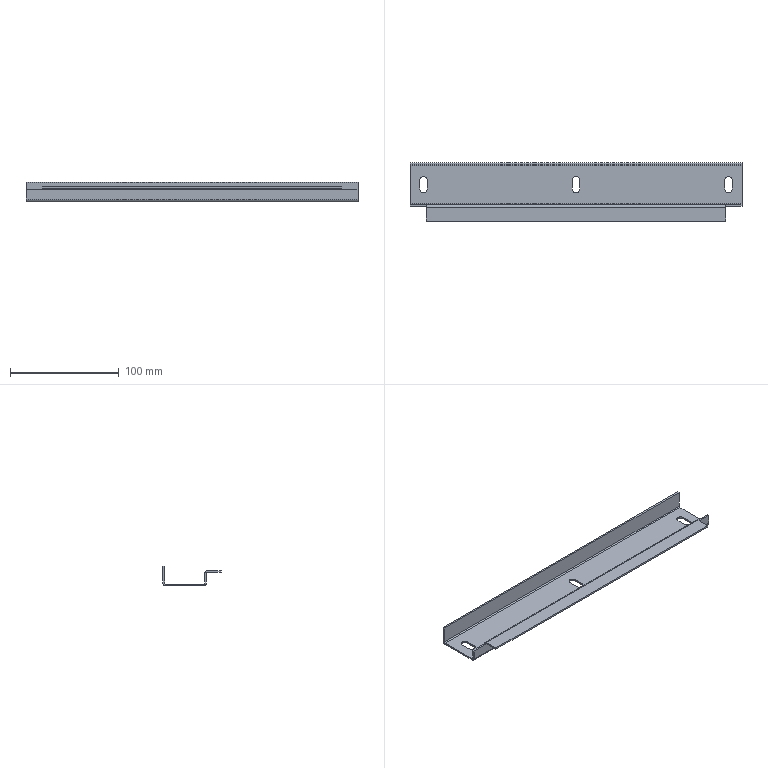Part | SolidWorks | features EdgeFlange 3, ICE 3, FlatPattern 1, SMBaseFlange 1, SheetMetal 1 | 1 solid | 42 faces | box 305 x 53.5 x 18 mm | volume 35601 mm3 | plane 30 | cylinder 12 | commonest cylinder face diameters 7 x6 2 x3 5 x3
STEP:
#1=CARTESIAN_POINT('',(137.5,-18.5,10.));
#2=VERTEX_POINT('',#1);
#3=CARTESIAN_POINT('',(137.5,-21.,12.5));
#4=VERTEX_POINT('',#3);
#5=CARTESIAN_POINT('',(137.5,-21.,10.));
#6=DIRECTION('',(1.,0.,0.));
#7=DIRECTION('',(0.,0.,1.));
#8=AXIS2_PLACEMENT_3D('',#5,#6,#7);
#9=CIRCLE('',#8,2.5);
#10=EDGE_CURVE('',#2,#4,#9,.T.);
#11=ORIENTED_EDGE('',*,*,#10,.F.);
#12=CARTESIAN_POINT('',(-137.5,-18.5,10.));
#13=VERTEX_POINT('',#12);
#14=CARTESIAN_POINT('',(-152.5,-18.5,10.));
#15=DIRECTION('',(1.,0.,0.));
#16=VECTOR('',#15,1000.);
#17=LINE('',#14,#16);
#18=EDGE_CURVE('',#13,#2,#17,.T.);
#19=ORIENTED_EDGE('',*,*,#18,.F.);
#20=CARTESIAN_POINT('',(-137.5,-21.,12.5));
#21=VERTEX_POINT('',#20);
#22=CARTESIAN_POINT('',(-137.5,-21.,10.));
#23=DIRECTION('',(1.,0.,0.));
#24=DIRECTION('',(0.,0.,1.));
#25=AXIS2_PLACEMENT_3D('',#22,#23,#24);
#26=CIRCLE('',#25,2.5);
#27=EDGE_CURVE('',#13,#21,#26,.T.);
#28=ORIENTED_EDGE('',*,*,#27,.T.);
#29=CARTESIAN_POINT('',(152.5,-21.,12.5));
#30=DIRECTION('',(1.,0.,0.));
#31=VECTOR('',#30,1000.);
#32=LINE('',#29,#31);
#33=EDGE_CURVE('',#21,#4,#32,.T.);
#34=ORIENTED_EDGE('',*,*,#33,.T.);
#35=EDGE_LOOP('',(#11,#19,#28,#34));
#36=FACE_OUTER_BOUND('',#35,.T.);
#37=CARTESIAN_POINT('',(-152.5,-21.,10.));
#38=DIRECTION('',(-1.,0.,0.));
#39=DIRECTION('',(0.,0.,1.));
#40=AXIS2_PLACEMENT_3D('',#37,#38,#39);
#41=CYLINDRICAL_SURFACE('',#40,2.5);
#42=ADVANCED_FACE('',(#36),#41,.T.);
#43=CARTESIAN_POINT('',(-137.5,-20.,10.));
#44=VERTEX_POINT('',#43);
#45=CARTESIAN_POINT('',(137.5,-20.,10.));
#46=VERTEX_POINT('',#45);
#47=CARTESIAN_POINT('',(-152.5,-20.,10.));
#48=DIRECTION('',(1.,0.,0.));
#49=VECTOR('',#48,1000.);
#50=LINE('',#47,#49);
#51=EDGE_CURVE('',#44,#46,#50,.T.);
#52=ORIENTED_EDGE('',*,*,#51,.T.);
#53=CARTESIAN_POINT('',(137.5,-21.,11.));
#54=VERTEX_POINT('',#53);
#55=CARTESIAN_POINT('',(137.5,-21.,10.));
#56=DIRECTION('',(1.,0.,0.));
#57=DIRECTION('',(0.,0.,1.));
#58=AXIS2_PLACEMENT_3D('',#55,#56,#57);
#59=CIRCLE('',#58,1.);
#60=EDGE_CURVE('',#46,#54,#59,.T.);
#61=ORIENTED_EDGE('',*,*,#60,.T.);
#62=CARTESIAN_POINT('',(-137.5,-21.,11.));
#63=VERTEX_POINT('',#62);
#64=CARTESIAN_POINT('',(152.5,-21.,11.));
#65=DIRECTION('',(-1.,0.,0.));
#66=VECTOR('',#65,1000.);
#67=LINE('',#64,#66);
#68=EDGE_CURVE('',#54,#63,#67,.T.);
#69=ORIENTED_EDGE('',*,*,#68,.T.);
#70=CARTESIAN_POINT('',(-137.5,-21.,10.));
#71=DIRECTION('',(1.,0.,0.));
#72=DIRECTION('',(0.,0.,1.));
#73=AXIS2_PLACEMENT_3D('',#70,#71,#72);
#74=CIRCLE('',#73,1.);
#75=EDGE_CURVE('',#44,#63,#74,.T.);
#76=ORIENTED_EDGE('',*,*,#75,.F.);
#77=EDGE_LOOP('',(#52,#61,#69,#76));
#78=FACE_OUTER_BOUND('',#77,.T.);
#79=CARTESIAN_POINT('',(-152.5,-21.,10.));
#80=DIRECTION('',(-1.,0.,0.));
#81=DIRECTION('',(0.,0.,1.));
#82=AXIS2_PLACEMENT_3D('',#79,#80,#81);
#83=CYLINDRICAL_SURFACE('',#82,1.);
#84=ADVANCED_FACE('',(#78),#83,.F.);
#85=CARTESIAN_POINT('',(-137.5,-33.5,12.5));
#86=VERTEX_POINT('',#85);
#87=CARTESIAN_POINT('',(137.5,-33.5,12.5));
#88=VERTEX_POINT('',#87);
#89=CARTESIAN_POINT('',(-152.5,-33.5,12.5));
#90=DIRECTION('',(1.,0.,0.));
#91=VECTOR('',#90,1000.);
#92=LINE('',#89,#91);
#93=EDGE_CURVE('',#86,#88,#92,.T.);
#94=ORIENTED_EDGE('',*,*,#93,.T.);
#95=CARTESIAN_POINT('',(137.5,-18.5,12.5));
#96=DIRECTION('',(0.,-1.,0.));
#97=VECTOR('',#96,1000.);
#98=LINE('',#95,#97);
#99=EDGE_CURVE('',#4,#88,#98,.T.);
#100=ORIENTED_EDGE('',*,*,#99,.F.);
#101=ORIENTED_EDGE('',*,*,#33,.F.);
#102=CARTESIAN_POINT('',(-137.5,-18.5,12.5));
#103=DIRECTION('',(0.,1.,0.));
#104=VECTOR('',#103,1000.);
#105=LINE('',#102,#104);
#106=EDGE_CURVE('',#86,#21,#105,.T.);
#107=ORIENTED_EDGE('',*,*,#106,.F.);
#108=EDGE_LOOP('',(#94,#100,#101,#107));
#109=FACE_OUTER_BOUND('',#108,.T.);
#110=CARTESIAN_POINT('',(-152.5,-20.,12.5));
#111=DIRECTION('',(0.,0.,-1.));
#112=DIRECTION('',(0.,1.,0.));
#113=AXIS2_PLACEMENT_3D('',#110,#111,#112);
#114=PLANE('',#113);
#115=ADVANCED_FACE('',(#109),#114,.F.);
#116=CARTESIAN_POINT('',(137.5,-33.5,11.));
#117=VERTEX_POINT('',#116);
#118=CARTESIAN_POINT('',(137.5,-20.,11.));
#119=DIRECTION('',(0.,1.,0.));
#120=VECTOR('',#119,1000.);
#121=LINE('',#118,#120);
#122=EDGE_CURVE('',#117,#54,#121,.T.);
#123=ORIENTED_EDGE('',*,*,#122,.F.);
#124=CARTESIAN_POINT('',(-137.5,-33.5,11.));
#125=VERTEX_POINT('',#124);
#126=CARTESIAN_POINT('',(152.5,-33.5,11.));
#127=DIRECTION('',(1.,0.,0.));
#128=VECTOR('',#127,1000.);
#129=LINE('',#126,#128);
#130=EDGE_CURVE('',#125,#117,#129,.T.);
#131=ORIENTED_EDGE('',*,*,#130,.F.);
#132=CARTESIAN_POINT('',(-137.5,-20.,11.));
#133=DIRECTION('',(0.,1.,0.));
#134=VECTOR('',#133,1000.);
#135=LINE('',#132,#134);
#136=EDGE_CURVE('',#125,#63,#135,.T.);
#137=ORIENTED_EDGE('',*,*,#136,.T.);
#138=ORIENTED_EDGE('',*,*,#68,.F.);
#139=EDGE_LOOP('',(#123,#131,#137,#138));
#140=FACE_OUTER_BOUND('',#139,.T.);
#141=CARTESIAN_POINT('',(-152.5,-20.,11.));
#142=DIRECTION('',(0.,0.,-1.));
#143=DIRECTION('',(0.,1.,0.));
#144=AXIS2_PLACEMENT_3D('',#141,#142,#143);
#145=PLANE('',#144);
#146=ADVANCED_FACE('',(#140),#145,.T.);
#147=ORIENTED_EDGE('',*,*,#130,.T.);
#148=CARTESIAN_POINT('',(137.5,-33.5,10.));
#149=DIRECTION('',(0.,0.,-1.));
#150=VECTOR('',#149,1000.);
#151=LINE('',#148,#150);
#152=EDGE_CURVE('',#88,#117,#151,.T.);
#153=ORIENTED_EDGE('',*,*,#152,.F.);
#154=ORIENTED_EDGE('',*,*,#93,.F.);
#155=CARTESIAN_POINT('',(-137.5,-33.5,12.5));
#156=DIRECTION('',(0.,0.,1.));
#157=VECTOR('',#156,1000.);
#158=LINE('',#155,#157);
#159=EDGE_CURVE('',#125,#86,#158,.T.);
#160=ORIENTED_EDGE('',*,*,#159,.F.);
#161=EDGE_LOOP('',(#147,#153,#154,#160));
#162=FACE_OUTER_BOUND('',#161,.T.);
#163=CARTESIAN_POINT('',(152.5,-33.5,12.5));
#164=DIRECTION('',(0.,1.,0.));
#165=DIRECTION('',(0.,0.,1.));
#166=AXIS2_PLACEMENT_3D('',#163,#164,#165);
#167=PLANE('',#166);
#168=ADVANCED_FACE('',(#162),#167,.F.);
#169=CARTESIAN_POINT('',(152.5,-20.,10.));
#170=VERTEX_POINT('',#169);
#171=CARTESIAN_POINT('',(152.5,-18.5,10.));
#172=VERTEX_POINT('',#171);
#173=CARTESIAN_POINT('',(152.5,-20.,10.));
#174=DIRECTION('',(0.,1.,0.));
#175=VECTOR('',#174,1000.);
#176=LINE('',#173,#175);
#177=EDGE_CURVE('',#170,#172,#176,.T.);
#178=ORIENTED_EDGE('',*,*,#177,.F.);
#179=CARTESIAN_POINT('',(152.5,-20.,1.));
#180=VERTEX_POINT('',#179);
#181=CARTESIAN_POINT('',(152.5,-20.,0.));
#182=DIRECTION('',(0.,0.,1.));
#183=VECTOR('',#182,1000.);
#184=LINE('',#181,#183);
#185=EDGE_CURVE('',#180,#170,#184,.T.);
#186=ORIENTED_EDGE('',*,*,#185,.F.);
#187=CARTESIAN_POINT('',(152.5,-18.5,1.));
#188=VERTEX_POINT('',#187);
#189=CARTESIAN_POINT('',(152.5,-18.5,1.));
#190=DIRECTION('',(0.,-1.,0.));
#191=VECTOR('',#190,1000.);
#192=LINE('',#189,#191);
#193=EDGE_CURVE('',#188,#180,#192,.T.);
#194=ORIENTED_EDGE('',*,*,#193,.F.);
#195=CARTESIAN_POINT('',(152.5,-18.5,12.5));
#196=DIRECTION('',(0.,0.,1.));
#197=VECTOR('',#196,1000.);
#198=LINE('',#195,#197);
#199=EDGE_CURVE('',#188,#172,#198,.T.);
#200=ORIENTED_EDGE('',*,*,#199,.T.);
#201=EDGE_LOOP('',(#178,#186,#194,#200));
#202=FACE_OUTER_BOUND('',#201,.T.);
#203=CARTESIAN_POINT('',(152.5,-20.,12.5));
#204=DIRECTION('',(-1.,0.,0.));
#205=DIRECTION('',(0.,0.,1.));
#206=AXIS2_PLACEMENT_3D('',#203,#204,#205);
#207=PLANE('',#206);
#208=ADVANCED_FACE('',(#202),#207,.F.);
#209=CARTESIAN_POINT('',(-152.5,-20.,10.));
#210=VERTEX_POINT('',#209);
#211=CARTESIAN_POINT('',(-152.5,-18.5,10.));
#212=VERTEX_POINT('',#211);
#213=CARTESIAN_POINT('',(-152.5,-20.,10.));
#214=DIRECTION('',(0.,1.,0.));
#215=VECTOR('',#214,1000.);
#216=LINE('',#213,#215);
#217=EDGE_CURVE('',#210,#212,#216,.T.);
#218=ORIENTED_EDGE('',*,*,#217,.T.);
#219=CARTESIAN_POINT('',(-152.5,-18.5,1.));
#220=VERTEX_POINT('',#219);
#221=CARTESIAN_POINT('',(-152.5,-18.5,0.));
#222=DIRECTION('',(0.,0.,-1.));
#223=VECTOR('',#222,1000.);
#224=LINE('',#221,#223);
#225=EDGE_CURVE('',#212,#220,#224,.T.);
#226=ORIENTED_EDGE('',*,*,#225,.T.);
#227=CARTESIAN_POINT('',(-152.5,-20.,1.));
#228=VERTEX_POINT('',#227);
#229=CARTESIAN_POINT('',(-152.5,-20.,1.));
#230=DIRECTION('',(0.,-1.,0.));
#231=VECTOR('',#230,1000.);
#232=LINE('',#229,#231);
#233=EDGE_CURVE('',#220,#228,#232,.T.);
#234=ORIENTED_EDGE('',*,*,#233,.T.);
#235=CARTESIAN_POINT('',(-152.5,-20.,0.));
#236=DIRECTION('',(0.,0.,-1.));
#237=VECTOR('',#236,1000.);
#238=LINE('',#235,#237);
#239=EDGE_CURVE('',#210,#228,#238,.T.);
#240=ORIENTED_EDGE('',*,*,#239,.F.);
#241=EDGE_LOOP('',(#218,#226,#234,#240));
#242=FACE_OUTER_BOUND('',#241,.T.);
#243=CARTESIAN_POINT('',(-152.5,-20.,0.));
#244=DIRECTION('',(1.,0.,0.));
#245=DIRECTION('',(0.,0.,-1.));
#246=AXIS2_PLACEMENT_3D('',#243,#244,#245);
#247=PLANE('',#246);
#248=ADVANCED_FACE('',(#242),#247,.F.);
#249=CARTESIAN_POINT('',(-152.5,-20.,10.));
#250=DIRECTION('',(1.,0.,0.));
#251=VECTOR('',#250,1000.);
#252=LINE('',#249,#251);
#253=EDGE_CURVE('',#210,#44,#252,.T.);
#254=ORIENTED_EDGE('',*,*,#253,.F.);
#255=ORIENTED_EDGE('',*,*,#239,.T.);
#256=CARTESIAN_POINT('',(-152.5,-20.,1.));
#257=DIRECTION('',(-1.,0.,0.));
#258=VECTOR('',#257,1000.);
#259=LINE('',#256,#258);
#260=EDGE_CURVE('',#180,#228,#259,.T.);
#261=ORIENTED_EDGE('',*,*,#260,.F.);
#262=ORIENTED_EDGE('',*,*,#185,.T.);
#263=CARTESIAN_POINT('',(152.5,-20.,10.));
#264=DIRECTION('',(-1.,0.,0.));
#265=VECTOR('',#264,1000.);
#266=LINE('',#263,#265);
#267=EDGE_CURVE('',#170,#46,#266,.T.);
#268=ORIENTED_EDGE('',*,*,#267,.T.);
#269=ORIENTED_EDGE('',*,*,#51,.F.);
#270=EDGE_LOOP('',(#254,#255,#261,#262,#268,#269));
#271=FACE_OUTER_BOUND('',#270,.T.);
#272=CARTESIAN_POINT('',(152.5,-20.,0.));
#273=DIRECTION('',(0.,1.,0.));
#274=DIRECTION('',(0.,0.,1.));
#275=AXIS2_PLACEMENT_3D('',#272,#273,#274);
#276=PLANE('',#275);
#277=ADVANCED_FACE('',(#271),#276,.F.);
#278=ORIENTED_EDGE('',*,*,#225,.F.);
#279=CARTESIAN_POINT('',(-152.5,-18.5,10.));
#280=DIRECTION('',(1.,0.,0.));
#281=VECTOR('',#280,1000.);
#282=LINE('',#279,#281);
#283=EDGE_CURVE('',#212,#13,#282,.T.);
#284=ORIENTED_EDGE('',*,*,#283,.T.);
#285=ORIENTED_EDGE('',*,*,#18,.T.);
#286=CARTESIAN_POINT('',(137.5,-18.5,10.));
#287=DIRECTION('',(1.,0.,0.));
#288=VECTOR('',#287,1000.);
#289=LINE('',#286,#288);
#290=EDGE_CURVE('',#2,#172,#289,.T.);
#291=ORIENTED_EDGE('',*,*,#290,.T.);
#292=ORIENTED_EDGE('',*,*,#199,.F.);
#293=CARTESIAN_POINT('',(-152.5,-18.5,1.));
#294=DIRECTION('',(1.,0.,0.));
#295=VECTOR('',#294,1000.);
#296=LINE('',#293,#295);
#297=EDGE_CURVE('',#220,#188,#296,.T.);
#298=ORIENTED_EDGE('',*,*,#297,.F.);
#299=EDGE_LOOP('',(#278,#284,#285,#291,#292,#298));
#300=FACE_OUTER_BOUND('',#299,.T.);
#301=CARTESIAN_POINT('',(152.5,-18.5,0.));
#302=DIRECTION('',(0.,1.,0.));
#303=DIRECTION('',(0.,0.,1.));
#304=AXIS2_PLACEMENT_3D('',#301,#302,#303);
#305=PLANE('',#304);
#306=ADVANCED_FACE('',(#300),#305,.T.);
#307=CARTESIAN_POINT('',(143.5,4.,-1.5));
#308=VERTEX_POINT('',#307);
#309=CARTESIAN_POINT('',(143.5,-4.,-1.5));
#310=VERTEX_POINT('',#309);
#311=CARTESIAN_POINT('',(143.5,4.,-1.5));
#312=DIRECTION('',(0.,-1.,0.));
#313=VECTOR('',#312,1000.);
#314=LINE('',#311,#313);
#315=EDGE_CURVE('',#308,#310,#314,.T.);
#316=ORIENTED_EDGE('',*,*,#315,.F.);
#317=CARTESIAN_POINT('',(136.5,4.,-1.5));
#318=VERTEX_POINT('',#317);
#319=CARTESIAN_POINT('',(140.,4.,-1.5));
#320=DIRECTION('',(0.,0.,-1.));
#321=DIRECTION('',(-1.,0.,0.));
#322=AXIS2_PLACEMENT_3D('',#319,#320,#321);
#323=CIRCLE('',#322,3.5);
#324=EDGE_CURVE('',#318,#308,#323,.T.);
#325=ORIENTED_EDGE('',*,*,#324,.F.);
#326=CARTESIAN_POINT('',(136.5,-4.,-1.5));
#327=VERTEX_POINT('',#326);
#328=CARTESIAN_POINT('',(136.5,4.,-1.5));
#329=DIRECTION('',(0.,1.,0.));
#330=VECTOR('',#329,1000.);
#331=LINE('',#328,#330);
#332=EDGE_CURVE('',#327,#318,#331,.T.);
#333=ORIENTED_EDGE('',*,*,#332,.F.);
#334=CARTESIAN_POINT('',(140.,-4.,-1.5));
#335=DIRECTION('',(0.,0.,-1.));
#336=DIRECTION('',(-1.,0.,0.));
#337=AXIS2_PLACEMENT_3D('',#334,#335,#336);
#338=CIRCLE('',#337,3.5);
#339=EDGE_CURVE('',#310,#327,#338,.T.);
#340=ORIENTED_EDGE('',*,*,#339,.F.);
#341=EDGE_LOOP('',(#316,#325,#333,#340));
#342=FACE_BOUND('',#341,.T.);
#343=CARTESIAN_POINT('',(-136.5,4.,-1.5));
#344=VERTEX_POINT('',#343);
#345=CARTESIAN_POINT('',(-136.5,-4.,-1.5));
#346=VERTEX_POINT('',#345);
#347=CARTESIAN_POINT('',(-136.5,4.,-1.5));
#348=DIRECTION('',(0.,-1.,0.));
#349=VECTOR('',#348,1000.);
#350=LINE('',#347,#349);
#351=EDGE_CURVE('',#344,#346,#350,.T.);
#352=ORIENTED_EDGE('',*,*,#351,.F.);
#353=CARTESIAN_POINT('',(-143.5,4.,-1.5));
#354=VERTEX_POINT('',#353);
#355=CARTESIAN_POINT('',(-140.,4.,-1.5));
#356=DIRECTION('',(0.,0.,-1.));
#357=DIRECTION('',(-1.,0.,0.));
#358=AXIS2_PLACEMENT_3D('',#355,#356,#357);
#359=CIRCLE('',#358,3.5);
#360=EDGE_CURVE('',#354,#344,#359,.T.);
#361=ORIENTED_EDGE('',*,*,#360,.F.);
#362=CARTESIAN_POINT('',(-143.5,-4.,-1.5));
#363=VERTEX_POINT('',#362);
#364=CARTESIAN_POINT('',(-143.5,4.,-1.5));
#365=DIRECTION('',(0.,1.,0.));
#366=VECTOR('',#365,1000.);
#367=LINE('',#364,#366);
#368=EDGE_CURVE('',#363,#354,#367,.T.);
#369=ORIENTED_EDGE('',*,*,#368,.F.);
#370=CARTESIAN_POINT('',(-140.,-4.,-1.5));
#371=DIRECTION('',(0.,0.,-1.));
#372=DIRECTION('',(-1.,0.,0.));
#373=AXIS2_PLACEMENT_3D('',#370,#371,#372);
#374=CIRCLE('',#373,3.5);
#375=EDGE_CURVE('',#346,#363,#374,.T.);
#376=ORIENTED_EDGE('',*,*,#375,.F.);
#377=EDGE_LOOP('',(#352,#361,#369,#376));
#378=FACE_BOUND('',#377,.T.);
#379=CARTESIAN_POINT('',(3.5,4.,-1.5));
#380=VERTEX_POINT('',#379);
#381=CARTESIAN_POINT('',(3.5,-4.,-1.5));
#382=VERTEX_POINT('',#381);
#383=CARTESIAN_POINT('',(3.5,4.,-1.5));
#384=DIRECTION('',(0.,-1.,0.));
#385=VECTOR('',#384,1000.);
#386=LINE('',#383,#385);
#387=EDGE_CURVE('',#380,#382,#386,.T.);
#388=ORIENTED_EDGE('',*,*,#387,.F.);
#389=CARTESIAN_POINT('',(-3.5,4.,-1.5));
#390=VERTEX_POINT('',#389);
#391=CARTESIAN_POINT('',(0.,4.,-1.5));
#392=DIRECTION('',(0.,0.,-1.));
#393=DIRECTION('',(-1.,0.,0.));
#394=AXIS2_PLACEMENT_3D('',#391,#392,#393);
#395=CIRCLE('',#394,3.5);
#396=EDGE_CURVE('',#390,#380,#395,.T.);
#397=ORIENTED_EDGE('',*,*,#396,.F.);
#398=CARTESIAN_POINT('',(-3.5,-4.,-1.5));
#399=VERTEX_POINT('',#398);
#400=CARTESIAN_POINT('',(-3.5,4.,-1.5));
#401=DIRECTION('',(0.,1.,0.));
#402=VECTOR('',#401,1000.);
#403=LINE('',#400,#402);
#404=EDGE_CURVE('',#399,#390,#403,.T.);
#405=ORIENTED_EDGE('',*,*,#404,.F.);
#406=CARTESIAN_POINT('',(0.,-4.,-1.5));
#407=DIRECTION('',(0.,0.,-1.));
#408=DIRECTION('',(-1.,0.,0.));
#409=AXIS2_PLACEMENT_3D('',#406,#407,#408);
#410=CIRCLE('',#409,3.5);
#411=EDGE_CURVE('',#382,#399,#410,.T.);
#412=ORIENTED_EDGE('',*,*,#411,.F.);
#413=EDGE_LOOP('',(#388,#397,#405,#412));
#414=FACE_BOUND('',#413,.T.);
#415=CARTESIAN_POINT('',(152.5,-17.5,-1.5));
#416=VERTEX_POINT('',#415);
#417=CARTESIAN_POINT('',(-152.5,-17.5,-1.5));
#418=VERTEX_POINT('',#417);
#419=CARTESIAN_POINT('',(152.5,-17.5,-1.5));
#420=DIRECTION('',(-1.,0.,0.));
#421=VECTOR('',#420,1000.);
#422=LINE('',#419,#421);
#423=EDGE_CURVE('',#416,#418,#422,.T.);
#424=ORIENTED_EDGE('',*,*,#423,.T.);
#425=CARTESIAN_POINT('',(-152.5,17.5,-1.5));
#426=VERTEX_POINT('',#425);
#427=CARTESIAN_POINT('',(-152.5,20.,-1.5));
#428=DIRECTION('',(0.,-1.,0.));
#429=VECTOR('',#428,1000.);
#430=LINE('',#427,#429);
#431=EDGE_CURVE('',#426,#418,#430,.T.);
#432=ORIENTED_EDGE('',*,*,#431,.F.);
#433=CARTESIAN_POINT('',(152.5,17.5,-1.5));
#434=VERTEX_POINT('',#433);
#435=CARTESIAN_POINT('',(-152.5,17.5,-1.5));
#436=DIRECTION('',(1.,0.,0.));
#437=VECTOR('',#436,1000.);
#438=LINE('',#435,#437);
#439=EDGE_CURVE('',#426,#434,#438,.T.);
#440=ORIENTED_EDGE('',*,*,#439,.T.);
#441=CARTESIAN_POINT('',(152.5,20.,-1.5));
#442=DIRECTION('',(0.,1.,0.));
#443=VECTOR('',#442,1000.);
#444=LINE('',#441,#443);
#445=EDGE_CURVE('',#416,#434,#444,.T.);
#446=ORIENTED_EDGE('',*,*,#445,.F.);
#447=EDGE_LOOP('',(#424,#432,#440,#446));
#448=FACE_OUTER_BOUND('',#447,.T.);
#449=CARTESIAN_POINT('',(152.5,-20.,-1.5));
#450=DIRECTION('',(0.,0.,1.));
#451=DIRECTION('',(1.,0.,0.));
#452=AXIS2_PLACEMENT_3D('',#449,#450,#451);
#453=PLANE('',#452);
#454=ADVANCED_FACE('',(#342,#378,#414,#448),#453,.F.);
#455=CARTESIAN_POINT('',(143.5,4.,0.));
#456=VERTEX_POINT('',#455);
#457=CARTESIAN_POINT('',(136.5,4.,0.));
#458=VERTEX_POINT('',#457);
#459=CARTESIAN_POINT('',(140.,4.,0.));
#460=DIRECTION('',(0.,0.,1.));
#461=DIRECTION('',(1.,0.,0.));
#462=AXIS2_PLACEMENT_3D('',#459,#460,#461);
#463=CIRCLE('',#462,3.5);
#464=EDGE_CURVE('',#456,#458,#463,.T.);
#465=ORIENTED_EDGE('',*,*,#464,.F.);
#466=CARTESIAN_POINT('',(143.5,-4.,0.));
#467=VERTEX_POINT('',#466);
#468=CARTESIAN_POINT('',(143.5,-20.,0.));
#469=DIRECTION('',(0.,1.,0.));
#470=VECTOR('',#469,1000.);
#471=LINE('',#468,#470);
#472=EDGE_CURVE('',#467,#456,#471,.T.);
#473=ORIENTED_EDGE('',*,*,#472,.F.);
#474=CARTESIAN_POINT('',(136.5,-4.,0.));
#475=VERTEX_POINT('',#474);
#476=CARTESIAN_POINT('',(140.,-4.,0.));
#477=DIRECTION('',(0.,0.,1.));
#478=DIRECTION('',(1.,0.,0.));
#479=AXIS2_PLACEMENT_3D('',#476,#477,#478);
#480=CIRCLE('',#479,3.5);
#481=EDGE_CURVE('',#475,#467,#480,.T.);
#482=ORIENTED_EDGE('',*,*,#481,.F.);
#483=CARTESIAN_POINT('',(136.5,-20.,0.));
#484=DIRECTION('',(0.,-1.,0.));
#485=VECTOR('',#484,1000.);
#486=LINE('',#483,#485);
#487=EDGE_CURVE('',#458,#475,#486,.T.);
#488=ORIENTED_EDGE('',*,*,#487,.F.);
#489=EDGE_LOOP('',(#465,#473,#482,#488));
#490=FACE_BOUND('',#489,.T.);
#491=CARTESIAN_POINT('',(-136.5,4.,0.));
#492=VERTEX_POINT('',#491);
#493=CARTESIAN_POINT('',(-143.5,4.,0.));
#494=VERTEX_POINT('',#493);
#495=CARTESIAN_POINT('',(-140.,4.,0.));
#496=DIRECTION('',(0.,0.,1.));
#497=DIRECTION('',(1.,0.,0.));
#498=AXIS2_PLACEMENT_3D('',#495,#496,#497);
#499=CIRCLE('',#498,3.5);
#500=EDGE_CURVE('',#492,#494,#499,.T.);
#501=ORIENTED_EDGE('',*,*,#500,.F.);
#502=CARTESIAN_POINT('',(-136.5,-4.,0.));
#503=VERTEX_POINT('',#502);
#504=CARTESIAN_POINT('',(-136.5,-20.,0.));
#505=DIRECTION('',(0.,1.,0.));
#506=VECTOR('',#505,1000.);
#507=LINE('',#504,#506);
#508=EDGE_CURVE('',#503,#492,#507,.T.);
#509=ORIENTED_EDGE('',*,*,#508,.F.);
#510=CARTESIAN_POINT('',(-143.5,-4.,0.));
#511=VERTEX_POINT('',#510);
#512=CARTESIAN_POINT('',(-140.,-4.,0.));
#513=DIRECTION('',(0.,0.,1.));
#514=DIRECTION('',(1.,0.,0.));
#515=AXIS2_PLACEMENT_3D('',#512,#513,#514);
#516=CIRCLE('',#515,3.5);
#517=EDGE_CURVE('',#511,#503,#516,.T.);
#518=ORIENTED_EDGE('',*,*,#517,.F.);
#519=CARTESIAN_POINT('',(-143.5,-20.,0.));
#520=DIRECTION('',(0.,-1.,0.));
#521=VECTOR('',#520,1000.);
#522=LINE('',#519,#521);
#523=EDGE_CURVE('',#494,#511,#522,.T.);
#524=ORIENTED_EDGE('',*,*,#523,.F.);
#525=EDGE_LOOP('',(#501,#509,#518,#524));
#526=FACE_BOUND('',#525,.T.);
#527=CARTESIAN_POINT('',(3.5,4.,0.));
#528=VERTEX_POINT('',#527);
#529=CARTESIAN_POINT('',(-3.5,4.,0.));
#530=VERTEX_POINT('',#529);
#531=CARTESIAN_POINT('',(0.,4.,0.));
#532=DIRECTION('',(0.,0.,1.));
#533=DIRECTION('',(1.,0.,0.));
#534=AXIS2_PLACEMENT_3D('',#531,#532,#533);
#535=CIRCLE('',#534,3.5);
#536=EDGE_CURVE('',#528,#530,#535,.T.);
#537=ORIENTED_EDGE('',*,*,#536,.F.);
#538=CARTESIAN_POINT('',(3.5,-4.,0.));
#539=VERTEX_POINT('',#538);
#540=CARTESIAN_POINT('',(3.5,-20.,0.));
#541=DIRECTION('',(0.,1.,0.));
#542=VECTOR('',#541,1000.);
#543=LINE('',#540,#542);
#544=EDGE_CURVE('',#539,#528,#543,.T.);
#545=ORIENTED_EDGE('',*,*,#544,.F.);
#546=CARTESIAN_POINT('',(-3.5,-4.,0.));
#547=VERTEX_POINT('',#546);
#548=CARTESIAN_POINT('',(0.,-4.,0.));
#549=DIRECTION('',(0.,0.,1.));
#550=DIRECTION('',(1.,0.,0.));
#551=AXIS2_PLACEMENT_3D('',#548,#549,#550);
#552=CIRCLE('',#551,3.5);
#553=EDGE_CURVE('',#547,#539,#552,.T.);
#554=ORIENTED_EDGE('',*,*,#553,.F.);
#555=CARTESIAN_POINT('',(-3.5,-20.,0.));
#556=DIRECTION('',(0.,-1.,0.));
#557=VECTOR('',#556,1000.);
#558=LINE('',#555,#557);
#559=EDGE_CURVE('',#530,#547,#558,.T.);
#560=ORIENTED_EDGE('',*,*,#559,.F.);
#561=EDGE_LOOP('',(#537,#545,#554,#560));
#562=FACE_BOUND('',#561,.T.);
#563=CARTESIAN_POINT('',(-152.5,17.5,0.));
#564=VERTEX_POINT('',#563);
#565=CARTESIAN_POINT('',(-152.5,-17.5,0.));
#566=VERTEX_POINT('',#565);
#567=CARTESIAN_POINT('',(-152.5,20.,0.));
#568=DIRECTION('',(0.,-1.,0.));
#569=VECTOR('',#568,1000.);
#570=LINE('',#567,#569);
#571=EDGE_CURVE('',#564,#566,#570,.T.);
#572=ORIENTED_EDGE('',*,*,#571,.T.);
#573=CARTESIAN_POINT('',(152.5,-17.5,0.));
#574=VERTEX_POINT('',#573);
#575=CARTESIAN_POINT('',(152.5,-17.5,0.));
#576=DIRECTION('',(-1.,0.,0.));
#577=VECTOR('',#576,1000.);
#578=LINE('',#575,#577);
#579=EDGE_CURVE('',#574,#566,#578,.T.);
#580=ORIENTED_EDGE('',*,*,#579,.F.);
#581=CARTESIAN_POINT('',(152.5,17.5,0.));
#582=VERTEX_POINT('',#581);
#583=CARTESIAN_POINT('',(152.5,20.,0.));
#584=DIRECTION('',(0.,1.,0.));
#585=VECTOR('',#584,1000.);
#586=LINE('',#583,#585);
#587=EDGE_CURVE('',#574,#582,#586,.T.);
#588=ORIENTED_EDGE('',*,*,#587,.T.);
#589=CARTESIAN_POINT('',(-152.5,17.5,0.));
#590=DIRECTION('',(1.,0.,0.));
#591=VECTOR('',#590,1000.);
#592=LINE('',#589,#591);
#593=EDGE_CURVE('',#564,#582,#592,.T.);
#594=ORIENTED_EDGE('',*,*,#593,.F.);
#595=EDGE_LOOP('',(#572,#580,#588,#594));
#596=FACE_OUTER_BOUND('',#595,.T.);
#597=CARTESIAN_POINT('',(152.5,-20.,0.));
#598=DIRECTION('',(0.,0.,1.));
#599=DIRECTION('',(1.,0.,0.));
#600=AXIS2_PLACEMENT_3D('',#597,#598,#599);
#601=PLANE('',#600);
#602=ADVANCED_FACE('',(#490,#526,#562,#596),#601,.T.);
#603=ORIENTED_EDGE('',*,*,#587,.F.);
#604=CARTESIAN_POINT('',(152.5,-17.5,0.));
#605=DIRECTION('',(0.,0.,-1.));
#606=VECTOR('',#605,1000.);
#607=LINE('',#604,#606);
#608=EDGE_CURVE('',#574,#416,#607,.T.);
#609=ORIENTED_EDGE('',*,*,#608,.T.);
#610=ORIENTED_EDGE('',*,*,#445,.T.);
#611=CARTESIAN_POINT('',(152.5,17.5,0.));
#612=DIRECTION('',(0.,0.,-1.));
#613=VECTOR('',#612,1000.);
#614=LINE('',#611,#613);
#615=EDGE_CURVE('',#582,#434,#614,.T.);
#616=ORIENTED_EDGE('',*,*,#615,.F.);
#617=EDGE_LOOP('',(#603,#609,#610,#616));
#618=FACE_OUTER_BOUND('',#617,.T.);
#619=CARTESIAN_POINT('',(152.5,20.,-1.5));
#620=DIRECTION('',(1.,0.,0.));
#621=DIRECTION('',(0.,0.,-1.));
#622=AXIS2_PLACEMENT_3D('',#619,#620,#621);
#623=PLANE('',#622);
#624=ADVANCED_FACE('',(#618),#623,.T.);
#625=CARTESIAN_POINT('',(-152.5,-17.5,0.));
#626=DIRECTION('',(0.,0.,-1.));
#627=VECTOR('',#626,1000.);
#628=LINE('',#625,#627);
#629=EDGE_CURVE('',#566,#418,#628,.T.);
#630=ORIENTED_EDGE('',*,*,#629,.F.);
#631=ORIENTED_EDGE('',*,*,#571,.F.);
#632=CARTESIAN_POINT('',(-152.5,17.5,0.));
#633=DIRECTION('',(0.,0.,-1.));
#634=VECTOR('',#633,1000.);
#635=LINE('',#632,#634);
#636=EDGE_CURVE('',#564,#426,#635,.T.);
#637=ORIENTED_EDGE('',*,*,#636,.T.);
#638=ORIENTED_EDGE('',*,*,#431,.T.);
#639=EDGE_LOOP('',(#630,#631,#637,#638));
#640=FACE_OUTER_BOUND('',#639,.T.);
#641=CARTESIAN_POINT('',(-152.5,20.,-1.5));
#642=DIRECTION('',(-1.,0.,0.));
#643=DIRECTION('',(0.,0.,1.));
#644=AXIS2_PLACEMENT_3D('',#641,#642,#643);
#645=PLANE('',#644);
#646=ADVANCED_FACE('',(#640),#645,.T.);
#647=CARTESIAN_POINT('',(152.5,18.5,1.));
#648=VERTEX_POINT('',#647);
#649=CARTESIAN_POINT('',(152.5,20.,1.));
#650=VERTEX_POINT('',#649);
#651=CARTESIAN_POINT('',(152.5,20.,1.));
#652=DIRECTION('',(0.,1.,0.));
#653=VECTOR('',#652,1000.);
#654=LINE('',#651,#653);
#655=EDGE_CURVE('',#648,#650,#654,.T.);
#656=ORIENTED_EDGE('',*,*,#655,.F.);
#657=CARTESIAN_POINT('',(152.5,17.5,1.));
#658=DIRECTION('',(1.,0.,0.));
#659=DIRECTION('',(0.,0.,1.));
#660=AXIS2_PLACEMENT_3D('',#657,#658,#659);
#661=CIRCLE('',#660,1.);
#662=EDGE_CURVE('',#582,#648,#661,.T.);
#663=ORIENTED_EDGE('',*,*,#662,.F.);
#664=ORIENTED_EDGE('',*,*,#615,.T.);
#665=CARTESIAN_POINT('',(152.5,17.5,1.));
#666=DIRECTION('',(1.,0.,0.));
#667=DIRECTION('',(0.,0.,1.));
#668=AXIS2_PLACEMENT_3D('',#665,#666,#667);
#669=CIRCLE('',#668,2.5);
#670=EDGE_CURVE('',#434,#650,#669,.T.);
#671=ORIENTED_EDGE('',*,*,#670,.T.);
#672=EDGE_LOOP('',(#656,#663,#664,#671));
#673=FACE_OUTER_BOUND('',#672,.T.);
#674=CARTESIAN_POINT('',(152.5,17.5,1.));
#675=DIRECTION('',(1.,0.,0.));
#676=DIRECTION('',(0.,0.,-1.));
#677=AXIS2_PLACEMENT_3D('',#674,#675,#676);
#678=PLANE('',#677);
#679=ADVANCED_FACE('',(#673),#678,.T.);
#680=ORIENTED_EDGE('',*,*,#439,.F.);
#681=CARTESIAN_POINT('',(-152.5,20.,1.));
#682=VERTEX_POINT('',#681);
#683=CARTESIAN_POINT('',(-152.5,17.5,1.));
#684=DIRECTION('',(-1.,0.,0.));
#685=DIRECTION('',(0.,0.,1.));
#686=AXIS2_PLACEMENT_3D('',#683,#684,#685);
#687=CIRCLE('',#686,2.5);
#688=EDGE_CURVE('',#682,#426,#687,.T.);
#689=ORIENTED_EDGE('',*,*,#688,.F.);
#690=CARTESIAN_POINT('',(152.5,20.,1.));
#691=DIRECTION('',(1.,0.,0.));
#692=VECTOR('',#691,1000.);
#693=LINE('',#690,#692);
#694=EDGE_CURVE('',#682,#650,#693,.T.);
#695=ORIENTED_EDGE('',*,*,#694,.T.);
#696=ORIENTED_EDGE('',*,*,#670,.F.);
#697=EDGE_LOOP('',(#680,#689,#695,#696));
#698=FACE_OUTER_BOUND('',#697,.T.);
#699=CARTESIAN_POINT('',(-152.5,17.5,1.));
#700=DIRECTION('',(-1.,0.,0.));
#701=DIRECTION('',(0.,1.,0.));
#702=AXIS2_PLACEMENT_3D('',#699,#700,#701);
#703=CYLINDRICAL_SURFACE('',#702,2.5);
#704=ADVANCED_FACE('',(#698),#703,.T.);
#705=CARTESIAN_POINT('',(-152.5,18.5,1.));
#706=VERTEX_POINT('',#705);
#707=CARTESIAN_POINT('',(-152.5,17.5,1.));
#708=DIRECTION('',(-1.,0.,0.));
#709=DIRECTION('',(0.,0.,1.));
#710=AXIS2_PLACEMENT_3D('',#707,#708,#709);
#711=CIRCLE('',#710,1.);
#712=EDGE_CURVE('',#706,#564,#711,.T.);
#713=ORIENTED_EDGE('',*,*,#712,.F.);
#714=CARTESIAN_POINT('',(-152.5,18.5,1.));
#715=DIRECTION('',(0.,1.,0.));
#716=VECTOR('',#715,1000.);
#717=LINE('',#714,#716);
#718=EDGE_CURVE('',#706,#682,#717,.T.);
#719=ORIENTED_EDGE('',*,*,#718,.T.);
#720=ORIENTED_EDGE('',*,*,#688,.T.);
#721=ORIENTED_EDGE('',*,*,#636,.F.);
#722=EDGE_LOOP('',(#713,#719,#720,#721));
#723=FACE_OUTER_BOUND('',#722,.T.);
#724=CARTESIAN_POINT('',(-152.5,17.5,1.));
#725=DIRECTION('',(1.,0.,0.));
#726=DIRECTION('',(0.,0.,-1.));
#727=AXIS2_PLACEMENT_3D('',#724,#725,#726);
#728=PLANE('',#727);
#729=ADVANCED_FACE('',(#723),#728,.F.);
#730=ORIENTED_EDGE('',*,*,#593,.T.);
#731=ORIENTED_EDGE('',*,*,#662,.T.);
#732=CARTESIAN_POINT('',(152.5,18.5,1.));
#733=DIRECTION('',(-1.,0.,0.));
#734=VECTOR('',#733,1000.);
#735=LINE('',#732,#734);
#736=EDGE_CURVE('',#648,#706,#735,.T.);
#737=ORIENTED_EDGE('',*,*,#736,.T.);
#738=ORIENTED_EDGE('',*,*,#712,.T.);
#739=EDGE_LOOP('',(#730,#731,#737,#738));
#740=FACE_OUTER_BOUND('',#739,.T.);
#741=CARTESIAN_POINT('',(-152.5,17.5,1.));
#742=DIRECTION('',(-1.,0.,0.));
#743=DIRECTION('',(0.,1.,0.));
#744=AXIS2_PLACEMENT_3D('',#741,#742,#743);
#745=CYLINDRICAL_SURFACE('',#744,1.);
#746=ADVANCED_FACE('',(#740),#745,.F.);
#747=ORIENTED_EDGE('',*,*,#655,.T.);
#748=CARTESIAN_POINT('',(152.5,20.,16.5));
#749=VERTEX_POINT('',#748);
#750=CARTESIAN_POINT('',(152.5,20.,16.5));
#751=DIRECTION('',(0.,0.,-1.));
#752=VECTOR('',#751,1000.);
#753=LINE('',#750,#752);
#754=EDGE_CURVE('',#749,#650,#753,.T.);
#755=ORIENTED_EDGE('',*,*,#754,.F.);
#756=CARTESIAN_POINT('',(152.5,18.5,16.5));
#757=VERTEX_POINT('',#756);
#758=CARTESIAN_POINT('',(152.5,20.,16.5));
#759=DIRECTION('',(0.,-1.,0.));
#760=VECTOR('',#759,1000.);
#761=LINE('',#758,#760);
#762=EDGE_CURVE('',#749,#757,#761,.T.);
#763=ORIENTED_EDGE('',*,*,#762,.T.);
#764=CARTESIAN_POINT('',(152.5,18.5,0.));
#765=DIRECTION('',(0.,0.,-1.));
#766=VECTOR('',#765,1000.);
#767=LINE('',#764,#766);
#768=EDGE_CURVE('',#757,#648,#767,.T.);
#769=ORIENTED_EDGE('',*,*,#768,.T.);
#770=EDGE_LOOP('',(#747,#755,#763,#769));
#771=FACE_OUTER_BOUND('',#770,.T.);
#772=CARTESIAN_POINT('',(152.5,20.,0.));
#773=DIRECTION('',(-1.,0.,0.));
#774=DIRECTION('',(0.,0.,1.));
#775=AXIS2_PLACEMENT_3D('',#772,#773,#774);
#776=PLANE('',#775);
#777=ADVANCED_FACE('',(#771),#776,.F.);
#778=ORIENTED_EDGE('',*,*,#718,.F.);
#779=CARTESIAN_POINT('',(-152.5,18.5,16.5));
#780=VERTEX_POINT('',#779);
#781=CARTESIAN_POINT('',(-152.5,18.5,16.5));
#782=DIRECTION('',(0.,0.,1.));
#783=VECTOR('',#782,1000.);
#784=LINE('',#781,#783);
#785=EDGE_CURVE('',#706,#780,#784,.T.);
#786=ORIENTED_EDGE('',*,*,#785,.T.);
#787=CARTESIAN_POINT('',(-152.5,20.,16.5));
#788=VERTEX_POINT('',#787);
#789=CARTESIAN_POINT('',(-152.5,20.,16.5));
#790=DIRECTION('',(0.,-1.,0.));
#791=VECTOR('',#790,1000.);
#792=LINE('',#789,#791);
#793=EDGE_CURVE('',#788,#780,#792,.T.);
#794=ORIENTED_EDGE('',*,*,#793,.F.);
#795=CARTESIAN_POINT('',(-152.5,20.,16.5));
#796=DIRECTION('',(0.,0.,1.));
#797=VECTOR('',#796,1000.);
#798=LINE('',#795,#797);
#799=EDGE_CURVE('',#682,#788,#798,.T.);
#800=ORIENTED_EDGE('',*,*,#799,.F.);
#801=EDGE_LOOP('',(#778,#786,#794,#800));
#802=FACE_OUTER_BOUND('',#801,.T.);
#803=CARTESIAN_POINT('',(-152.5,20.,16.5));
#804=DIRECTION('',(1.,0.,0.));
#805=DIRECTION('',(0.,0.,-1.));
#806=AXIS2_PLACEMENT_3D('',#803,#804,#805);
#807=PLANE('',#806);
#808=ADVANCED_FACE('',(#802),#807,.F.);
#809=ORIENTED_EDGE('',*,*,#694,.F.);
#810=ORIENTED_EDGE('',*,*,#799,.T.);
#811=CARTESIAN_POINT('',(152.5,20.,16.5));
#812=DIRECTION('',(1.,0.,0.));
#813=VECTOR('',#812,1000.);
#814=LINE('',#811,#813);
#815=EDGE_CURVE('',#788,#749,#814,.T.);
#816=ORIENTED_EDGE('',*,*,#815,.T.);
#817=ORIENTED_EDGE('',*,*,#754,.T.);
#818=EDGE_LOOP('',(#809,#810,#816,#817));
#819=FACE_OUTER_BOUND('',#818,.T.);
#820=CARTESIAN_POINT('',(152.5,20.,16.5));
#821=DIRECTION('',(0.,-1.,0.));
#822=DIRECTION('',(0.,0.,-1.));
#823=AXIS2_PLACEMENT_3D('',#820,#821,#822);
#824=PLANE('',#823);
#825=ADVANCED_FACE('',(#819),#824,.F.);
#826=ORIENTED_EDGE('',*,*,#785,.F.);
#827=ORIENTED_EDGE('',*,*,#736,.F.);
#828=ORIENTED_EDGE('',*,*,#768,.F.);
#829=CARTESIAN_POINT('',(152.5,18.5,16.5));
#830=DIRECTION('',(1.,0.,0.));
#831=VECTOR('',#830,1000.);
#832=LINE('',#829,#831);
#833=EDGE_CURVE('',#780,#757,#832,.T.);
#834=ORIENTED_EDGE('',*,*,#833,.F.);
#835=EDGE_LOOP('',(#826,#827,#828,#834));
#836=FACE_OUTER_BOUND('',#835,.T.);
#837=CARTESIAN_POINT('',(152.5,18.5,16.5));
#838=DIRECTION('',(0.,-1.,0.));
#839=DIRECTION('',(0.,0.,-1.));
#840=AXIS2_PLACEMENT_3D('',#837,#838,#839);
#841=PLANE('',#840);
#842=ADVANCED_FACE('',(#836),#841,.T.);
#843=ORIENTED_EDGE('',*,*,#833,.T.);
#844=ORIENTED_EDGE('',*,*,#762,.F.);
#845=ORIENTED_EDGE('',*,*,#815,.F.);
#846=ORIENTED_EDGE('',*,*,#793,.T.);
#847=EDGE_LOOP('',(#843,#844,#845,#846));
#848=FACE_OUTER_BOUND('',#847,.T.);
#849=CARTESIAN_POINT('',(152.5,20.,16.5));
#850=DIRECTION('',(0.,0.,-1.));
#851=DIRECTION('',(0.,1.,0.));
#852=AXIS2_PLACEMENT_3D('',#849,#850,#851);
#853=PLANE('',#852);
#854=ADVANCED_FACE('',(#848),#853,.F.);
#855=ORIENTED_EDGE('',*,*,#233,.F.);
#856=CARTESIAN_POINT('',(-152.5,-17.5,1.));
#857=DIRECTION('',(-1.,0.,0.));
#858=DIRECTION('',(0.,0.,-1.));
#859=AXIS2_PLACEMENT_3D('',#856,#857,#858);
#860=CIRCLE('',#859,1.);
#861=EDGE_CURVE('',#566,#220,#860,.T.);
#862=ORIENTED_EDGE('',*,*,#861,.F.);
#863=ORIENTED_EDGE('',*,*,#629,.T.);
#864=CARTESIAN_POINT('',(-152.5,-17.5,1.));
#865=DIRECTION('',(-1.,0.,0.));
#866=DIRECTION('',(0.,0.,-1.));
#867=AXIS2_PLACEMENT_3D('',#864,#865,#866);
#868=CIRCLE('',#867,2.5);
#869=EDGE_CURVE('',#418,#228,#868,.T.);
#870=ORIENTED_EDGE('',*,*,#869,.T.);
#871=EDGE_LOOP('',(#855,#862,#863,#870));
#872=FACE_OUTER_BOUND('',#871,.T.);
#873=CARTESIAN_POINT('',(-152.5,-17.5,1.));
#874=DIRECTION('',(-1.,0.,0.));
#875=DIRECTION('',(0.,0.,1.));
#876=AXIS2_PLACEMENT_3D('',#873,#874,#875);
#877=PLANE('',#876);
#878=ADVANCED_FACE('',(#872),#877,.T.);
#879=ORIENTED_EDGE('',*,*,#423,.F.);
#880=CARTESIAN_POINT('',(152.5,-17.5,1.));
#881=DIRECTION('',(1.,0.,0.));
#882=DIRECTION('',(0.,0.,-1.));
#883=AXIS2_PLACEMENT_3D('',#880,#881,#882);
#884=CIRCLE('',#883,2.5);
#885=EDGE_CURVE('',#180,#416,#884,.T.);
#886=ORIENTED_EDGE('',*,*,#885,.F.);
#887=ORIENTED_EDGE('',*,*,#260,.T.);
#888=ORIENTED_EDGE('',*,*,#869,.F.);
#889=EDGE_LOOP('',(#879,#886,#887,#888));
#890=FACE_OUTER_BOUND('',#889,.T.);
#891=CARTESIAN_POINT('',(152.5,-17.5,1.));
#892=DIRECTION('',(1.,0.,0.));
#893=DIRECTION('',(0.,-1.,0.));
#894=AXIS2_PLACEMENT_3D('',#891,#892,#893);
#895=CYLINDRICAL_SURFACE('',#894,2.5);
#896=ADVANCED_FACE('',(#890),#895,.T.);
#897=CARTESIAN_POINT('',(152.5,-17.5,1.));
#898=DIRECTION('',(1.,0.,0.));
#899=DIRECTION('',(0.,0.,-1.));
#900=AXIS2_PLACEMENT_3D('',#897,#898,#899);
#901=CIRCLE('',#900,1.);
#902=EDGE_CURVE('',#188,#574,#901,.T.);
#903=ORIENTED_EDGE('',*,*,#902,.F.);
#904=ORIENTED_EDGE('',*,*,#193,.T.);
#905=ORIENTED_EDGE('',*,*,#885,.T.);
#906=ORIENTED_EDGE('',*,*,#608,.F.);
#907=EDGE_LOOP('',(#903,#904,#905,#906));
#908=FACE_OUTER_BOUND('',#907,.T.);
#909=CARTESIAN_POINT('',(152.5,-17.5,1.));
#910=DIRECTION('',(-1.,0.,0.));
#911=DIRECTION('',(0.,0.,1.));
#912=AXIS2_PLACEMENT_3D('',#909,#910,#911);
#913=PLANE('',#912);
#914=ADVANCED_FACE('',(#908),#913,.F.);
#915=ORIENTED_EDGE('',*,*,#579,.T.);
#916=ORIENTED_EDGE('',*,*,#861,.T.);
#917=ORIENTED_EDGE('',*,*,#297,.T.);
#918=ORIENTED_EDGE('',*,*,#902,.T.);
#919=EDGE_LOOP('',(#915,#916,#917,#918));
#920=FACE_OUTER_BOUND('',#919,.T.);
#921=CARTESIAN_POINT('',(152.5,-17.5,1.));
#922=DIRECTION('',(1.,0.,0.));
#923=DIRECTION('',(0.,-1.,0.));
#924=AXIS2_PLACEMENT_3D('',#921,#922,#923);
#925=CYLINDRICAL_SURFACE('',#924,1.);
#926=ADVANCED_FACE('',(#920),#925,.F.);
#927=CARTESIAN_POINT('',(-137.5,-18.5,10.));
#928=DIRECTION('',(0.,-1.,0.));
#929=VECTOR('',#928,1000.);
#930=LINE('',#927,#929);
#931=EDGE_CURVE('',#13,#44,#930,.T.);
#932=ORIENTED_EDGE('',*,*,#931,.F.);
#933=ORIENTED_EDGE('',*,*,#283,.F.);
#934=ORIENTED_EDGE('',*,*,#217,.F.);
#935=ORIENTED_EDGE('',*,*,#253,.T.);
#936=EDGE_LOOP('',(#932,#933,#934,#935));
#937=FACE_OUTER_BOUND('',#936,.T.);
#938=CARTESIAN_POINT('',(-137.5,-18.5,10.));
#939=DIRECTION('',(0.,0.,-1.));
#940=DIRECTION('',(0.,1.,0.));
#941=AXIS2_PLACEMENT_3D('',#938,#939,#940);
#942=PLANE('',#941);
#943=ADVANCED_FACE('',(#937),#942,.F.);
#944=ORIENTED_EDGE('',*,*,#931,.T.);
#945=ORIENTED_EDGE('',*,*,#75,.T.);
#946=ORIENTED_EDGE('',*,*,#136,.F.);
#947=ORIENTED_EDGE('',*,*,#159,.T.);
#948=ORIENTED_EDGE('',*,*,#106,.T.);
#949=ORIENTED_EDGE('',*,*,#27,.F.);
#950=EDGE_LOOP('',(#944,#945,#946,#947,#948,#949));
#951=FACE_OUTER_BOUND('',#950,.T.);
#952=CARTESIAN_POINT('',(-137.5,-33.5,10.));
#953=DIRECTION('',(-1.,0.,0.));
#954=DIRECTION('',(0.,0.,1.));
#955=AXIS2_PLACEMENT_3D('',#952,#953,#954);
#956=PLANE('',#955);
#957=ADVANCED_FACE('',(#951),#956,.T.);
#958=ORIENTED_EDGE('',*,*,#10,.T.);
#959=ORIENTED_EDGE('',*,*,#99,.T.);
#960=ORIENTED_EDGE('',*,*,#152,.T.);
#961=ORIENTED_EDGE('',*,*,#122,.T.);
#962=ORIENTED_EDGE('',*,*,#60,.F.);
#963=CARTESIAN_POINT('',(137.5,-18.5,10.));
#964=DIRECTION('',(0.,1.,0.));
#965=VECTOR('',#964,1000.);
#966=LINE('',#963,#965);
#967=EDGE_CURVE('',#46,#2,#966,.T.);
#968=ORIENTED_EDGE('',*,*,#967,.T.);
#969=EDGE_LOOP('',(#958,#959,#960,#961,#962,#968));
#970=FACE_OUTER_BOUND('',#969,.T.);
#971=CARTESIAN_POINT('',(137.5,-33.5,10.));
#972=DIRECTION('',(-1.,0.,0.));
#973=DIRECTION('',(0.,0.,1.));
#974=AXIS2_PLACEMENT_3D('',#971,#972,#973);
#975=PLANE('',#974);
#976=ADVANCED_FACE('',(#970),#975,.F.);
#977=ORIENTED_EDGE('',*,*,#177,.T.);
#978=ORIENTED_EDGE('',*,*,#290,.F.);
#979=ORIENTED_EDGE('',*,*,#967,.F.);
#980=ORIENTED_EDGE('',*,*,#267,.F.);
#981=EDGE_LOOP('',(#977,#978,#979,#980));
#982=FACE_OUTER_BOUND('',#981,.T.);
#983=CARTESIAN_POINT('',(137.5,-18.5,10.));
#984=DIRECTION('',(0.,0.,-1.));
#985=DIRECTION('',(0.,1.,0.));
#986=AXIS2_PLACEMENT_3D('',#983,#984,#985);
#987=PLANE('',#986);
#988=ADVANCED_FACE('',(#982),#987,.F.);
#989=ORIENTED_EDGE('',*,*,#536,.T.);
#990=CARTESIAN_POINT('',(-3.5,4.,0.5));
#991=DIRECTION('',(0.,0.,-1.));
#992=VECTOR('',#991,1000.);
#993=LINE('',#990,#992);
#994=EDGE_CURVE('',#530,#390,#993,.T.);
#995=ORIENTED_EDGE('',*,*,#994,.T.);
#996=ORIENTED_EDGE('',*,*,#396,.T.);
#997=CARTESIAN_POINT('',(3.5,4.,0.5));
#998=DIRECTION('',(0.,0.,-1.));
#999=VECTOR('',#998,1000.);
#1000=LINE('',#997,#999);
#1001=EDGE_CURVE('',#528,#380,#1000,.T.);
#1002=ORIENTED_EDGE('',*,*,#1001,.F.);
#1003=EDGE_LOOP('',(#989,#995,#996,#1002));
#1004=FACE_OUTER_BOUND('',#1003,.T.);
#1005=CARTESIAN_POINT('',(0.,4.,0.5));
#1006=DIRECTION('',(0.,0.,-1.));
#1007=DIRECTION('',(-1.,0.,0.));
#1008=AXIS2_PLACEMENT_3D('',#1005,#1006,#1007);
#1009=CYLINDRICAL_SURFACE('',#1008,3.5);
#1010=ADVANCED_FACE('',(#1004),#1009,.F.);
#1011=ORIENTED_EDGE('',*,*,#559,.T.);
#1012=CARTESIAN_POINT('',(-3.5,-4.,0.5));
#1013=DIRECTION('',(0.,0.,-1.));
#1014=VECTOR('',#1013,1000.);
#1015=LINE('',#1012,#1014);
#1016=EDGE_CURVE('',#547,#399,#1015,.T.);
#1017=ORIENTED_EDGE('',*,*,#1016,.T.);
#1018=ORIENTED_EDGE('',*,*,#404,.T.);
#1019=ORIENTED_EDGE('',*,*,#994,.F.);
#1020=EDGE_LOOP('',(#1011,#1017,#1018,#1019));
#1021=FACE_OUTER_BOUND('',#1020,.T.);
#1022=CARTESIAN_POINT('',(-3.5,4.,0.5));
#1023=DIRECTION('',(-1.,0.,0.));
#1024=DIRECTION('',(0.,0.,1.));
#1025=AXIS2_PLACEMENT_3D('',#1022,#1023,#1024);
#1026=PLANE('',#1025);
#1027=ADVANCED_FACE('',(#1021),#1026,.F.);
#1028=ORIENTED_EDGE('',*,*,#553,.T.);
#1029=CARTESIAN_POINT('',(3.5,-4.,0.5));
#1030=DIRECTION('',(0.,0.,-1.));
#1031=VECTOR('',#1030,1000.);
#1032=LINE('',#1029,#1031);
#1033=EDGE_CURVE('',#539,#382,#1032,.T.);
#1034=ORIENTED_EDGE('',*,*,#1033,.T.);
#1035=ORIENTED_EDGE('',*,*,#411,.T.);
#1036=ORIENTED_EDGE('',*,*,#1016,.F.);
#1037=EDGE_LOOP('',(#1028,#1034,#1035,#1036));
#1038=FACE_OUTER_BOUND('',#1037,.T.);
#1039=CARTESIAN_POINT('',(0.,-4.,0.5));
#1040=DIRECTION('',(0.,0.,-1.));
#1041=DIRECTION('',(-1.,0.,0.));
#1042=AXIS2_PLACEMENT_3D('',#1039,#1040,#1041);
#1043=CYLINDRICAL_SURFACE('',#1042,3.5);
#1044=ADVANCED_FACE('',(#1038),#1043,.F.);
#1045=ORIENTED_EDGE('',*,*,#544,.T.);
#1046=ORIENTED_EDGE('',*,*,#1001,.T.);
#1047=ORIENTED_EDGE('',*,*,#387,.T.);
#1048=ORIENTED_EDGE('',*,*,#1033,.F.);
#1049=EDGE_LOOP('',(#1045,#1046,#1047,#1048));
#1050=FACE_OUTER_BOUND('',#1049,.T.);
#1051=CARTESIAN_POINT('',(3.5,4.,0.5));
#1052=DIRECTION('',(1.,0.,0.));
#1053=DIRECTION('',(0.,0.,-1.));
#1054=AXIS2_PLACEMENT_3D('',#1051,#1052,#1053);
#1055=PLANE('',#1054);
#1056=ADVANCED_FACE('',(#1050),#1055,.F.);
#1057=ORIENTED_EDGE('',*,*,#500,.T.);
#1058=CARTESIAN_POINT('',(-143.5,4.,0.5));
#1059=DIRECTION('',(0.,0.,-1.));
#1060=VECTOR('',#1059,1000.);
#1061=LINE('',#1058,#1060);
#1062=EDGE_CURVE('',#494,#354,#1061,.T.);
#1063=ORIENTED_EDGE('',*,*,#1062,.T.);
#1064=ORIENTED_EDGE('',*,*,#360,.T.);
#1065=CARTESIAN_POINT('',(-136.5,4.,0.5));
#1066=DIRECTION('',(0.,0.,-1.));
#1067=VECTOR('',#1066,1000.);
#1068=LINE('',#1065,#1067);
#1069=EDGE_CURVE('',#492,#344,#1068,.T.);
#1070=ORIENTED_EDGE('',*,*,#1069,.F.);
#1071=EDGE_LOOP('',(#1057,#1063,#1064,#1070));
#1072=FACE_OUTER_BOUND('',#1071,.T.);
#1073=CARTESIAN_POINT('',(-140.,4.,0.5));
#1074=DIRECTION('',(0.,0.,-1.));
#1075=DIRECTION('',(-1.,0.,0.));
#1076=AXIS2_PLACEMENT_3D('',#1073,#1074,#1075);
#1077=CYLINDRICAL_SURFACE('',#1076,3.5);
#1078=ADVANCED_FACE('',(#1072),#1077,.F.);
#1079=ORIENTED_EDGE('',*,*,#523,.T.);
#1080=CARTESIAN_POINT('',(-143.5,-4.,0.5));
#1081=DIRECTION('',(0.,0.,-1.));
#1082=VECTOR('',#1081,1000.);
#1083=LINE('',#1080,#1082);
#1084=EDGE_CURVE('',#511,#363,#1083,.T.);
#1085=ORIENTED_EDGE('',*,*,#1084,.T.);
#1086=ORIENTED_EDGE('',*,*,#368,.T.);
#1087=ORIENTED_EDGE('',*,*,#1062,.F.);
#1088=EDGE_LOOP('',(#1079,#1085,#1086,#1087));
#1089=FACE_OUTER_BOUND('',#1088,.T.);
#1090=CARTESIAN_POINT('',(-143.5,4.,0.5));
#1091=DIRECTION('',(-1.,0.,0.));
#1092=DIRECTION('',(0.,0.,1.));
#1093=AXIS2_PLACEMENT_3D('',#1090,#1091,#1092);
#1094=PLANE('',#1093);
#1095=ADVANCED_FACE('',(#1089),#1094,.F.);
#1096=ORIENTED_EDGE('',*,*,#517,.T.);
#1097=CARTESIAN_POINT('',(-136.5,-4.,0.5));
#1098=DIRECTION('',(0.,0.,-1.));
#1099=VECTOR('',#1098,1000.);
#1100=LINE('',#1097,#1099);
#1101=EDGE_CURVE('',#503,#346,#1100,.T.);
#1102=ORIENTED_EDGE('',*,*,#1101,.T.);
#1103=ORIENTED_EDGE('',*,*,#375,.T.);
#1104=ORIENTED_EDGE('',*,*,#1084,.F.);
#1105=EDGE_LOOP('',(#1096,#1102,#1103,#1104));
#1106=FACE_OUTER_BOUND('',#1105,.T.);
#1107=CARTESIAN_POINT('',(-140.,-4.,0.5));
#1108=DIRECTION('',(0.,0.,-1.));
#1109=DIRECTION('',(-1.,0.,0.));
#1110=AXIS2_PLACEMENT_3D('',#1107,#1108,#1109);
#1111=CYLINDRICAL_SURFACE('',#1110,3.5);
#1112=ADVANCED_FACE('',(#1106),#1111,.F.);
#1113=ORIENTED_EDGE('',*,*,#508,.T.);
#1114=ORIENTED_EDGE('',*,*,#1069,.T.);
#1115=ORIENTED_EDGE('',*,*,#351,.T.);
#1116=ORIENTED_EDGE('',*,*,#1101,.F.);
#1117=EDGE_LOOP('',(#1113,#1114,#1115,#1116));
#1118=FACE_OUTER_BOUND('',#1117,.T.);
#1119=CARTESIAN_POINT('',(-136.5,4.,0.5));
#1120=DIRECTION('',(1.,0.,0.));
#1121=DIRECTION('',(0.,0.,-1.));
#1122=AXIS2_PLACEMENT_3D('',#1119,#1120,#1121);
#1123=PLANE('',#1122);
#1124=ADVANCED_FACE('',(#1118),#1123,.F.);
#1125=ORIENTED_EDGE('',*,*,#464,.T.);
#1126=CARTESIAN_POINT('',(136.5,4.,0.5));
#1127=DIRECTION('',(0.,0.,-1.));
#1128=VECTOR('',#1127,1000.);
#1129=LINE('',#1126,#1128);
#1130=EDGE_CURVE('',#458,#318,#1129,.T.);
#1131=ORIENTED_EDGE('',*,*,#1130,.T.);
#1132=ORIENTED_EDGE('',*,*,#324,.T.);
#1133=CARTESIAN_POINT('',(143.5,4.,0.5));
#1134=DIRECTION('',(0.,0.,-1.));
#1135=VECTOR('',#1134,1000.);
#1136=LINE('',#1133,#1135);
#1137=EDGE_CURVE('',#456,#308,#1136,.T.);
#1138=ORIENTED_EDGE('',*,*,#1137,.F.);
#1139=EDGE_LOOP('',(#1125,#1131,#1132,#1138));
#1140=FACE_OUTER_BOUND('',#1139,.T.);
#1141=CARTESIAN_POINT('',(140.,4.,0.5));
#1142=DIRECTION('',(0.,0.,-1.));
#1143=DIRECTION('',(-1.,0.,0.));
#1144=AXIS2_PLACEMENT_3D('',#1141,#1142,#1143);
#1145=CYLINDRICAL_SURFACE('',#1144,3.5);
#1146=ADVANCED_FACE('',(#1140),#1145,.F.);
#1147=ORIENTED_EDGE('',*,*,#487,.T.);
#1148=CARTESIAN_POINT('',(136.5,-4.,0.5));
#1149=DIRECTION('',(0.,0.,-1.));
#1150=VECTOR('',#1149,1000.);
#1151=LINE('',#1148,#1150);
#1152=EDGE_CURVE('',#475,#327,#1151,.T.);
#1153=ORIENTED_EDGE('',*,*,#1152,.T.);
#1154=ORIENTED_EDGE('',*,*,#332,.T.);
#1155=ORIENTED_EDGE('',*,*,#1130,.F.);
#1156=EDGE_LOOP('',(#1147,#1153,#1154,#1155));
#1157=FACE_OUTER_BOUND('',#1156,.T.);
#1158=CARTESIAN_POINT('',(136.5,4.,0.5));
#1159=DIRECTION('',(-1.,0.,0.));
#1160=DIRECTION('',(0.,0.,1.));
#1161=AXIS2_PLACEMENT_3D('',#1158,#1159,#1160);
#1162=PLANE('',#1161);
#1163=ADVANCED_FACE('',(#1157),#1162,.F.);
#1164=ORIENTED_EDGE('',*,*,#481,.T.);
#1165=CARTESIAN_POINT('',(143.5,-4.,0.5));
#1166=DIRECTION('',(0.,0.,-1.));
#1167=VECTOR('',#1166,1000.);
#1168=LINE('',#1165,#1167);
#1169=EDGE_CURVE('',#467,#310,#1168,.T.);
#1170=ORIENTED_EDGE('',*,*,#1169,.T.);
#1171=ORIENTED_EDGE('',*,*,#339,.T.);
#1172=ORIENTED_EDGE('',*,*,#1152,.F.);
#1173=EDGE_LOOP('',(#1164,#1170,#1171,#1172));
#1174=FACE_OUTER_BOUND('',#1173,.T.);
#1175=CARTESIAN_POINT('',(140.,-4.,0.5));
#1176=DIRECTION('',(0.,0.,-1.));
#1177=DIRECTION('',(-1.,0.,0.));
#1178=AXIS2_PLACEMENT_3D('',#1175,#1176,#1177);
#1179=CYLINDRICAL_SURFACE('',#1178,3.5);
#1180=ADVANCED_FACE('',(#1174),#1179,.F.);
#1181=ORIENTED_EDGE('',*,*,#472,.T.);
#1182=ORIENTED_EDGE('',*,*,#1137,.T.);
#1183=ORIENTED_EDGE('',*,*,#315,.T.);
#1184=ORIENTED_EDGE('',*,*,#1169,.F.);
#1185=EDGE_LOOP('',(#1181,#1182,#1183,#1184));
#1186=FACE_OUTER_BOUND('',#1185,.T.);
#1187=CARTESIAN_POINT('',(143.5,4.,0.5));
#1188=DIRECTION('',(1.,0.,0.));
#1189=DIRECTION('',(0.,0.,-1.));
#1190=AXIS2_PLACEMENT_3D('',#1187,#1188,#1189);
#1191=PLANE('',#1190);
#1192=ADVANCED_FACE('',(#1186),#1191,.F.);
#1193=CLOSED_SHELL('',(#42,#84,#115,#146,#168,#208,#248,#277,#306,#454,#602,#624,#646,#679,#704,#729,#746,#777,#808,#825,#842,#854,#878,#896,#914,#926,#943,#957,#976,#988,#1010,#1027,#1044,#1056,#1078,#1095,#1112,#1124,#1146,#1163,#1180,#1192));
#1194=MANIFOLD_SOLID_BREP('',#1193);
#1195=CARTESIAN_POINT('',(0.,0.,0.));
#1196=DIRECTION('',(0.,0.,1.));
#1197=DIRECTION('',(1.,0.,0.));
#1198=AXIS2_PLACEMENT_3D('',#1195,#1196,#1197);
#1199=(LENGTH_UNIT()NAMED_UNIT(*)SI_UNIT(.MILLI.,.METRE.));
#1200=UNCERTAINTY_MEASURE_WITH_UNIT(LENGTH_MEASURE(0.00001),#1199,'','');
#1201=(NAMED_UNIT(*)PLANE_ANGLE_UNIT()SI_UNIT($,.RADIAN.));
#1202=(NAMED_UNIT(*)SI_UNIT($,.STERADIAN.)SOLID_ANGLE_UNIT());
#1203=(GEOMETRIC_REPRESENTATION_CONTEXT(3)GLOBAL_UNCERTAINTY_ASSIGNED_CONTEXT((#1200))GLOBAL_UNIT_ASSIGNED_CONTEXT((#1199,#1201,#1202))REPRESENTATION_CONTEXT('',''));
#1204=ADVANCED_BREP_SHAPE_REPRESENTATION('',(#1194,#1198),#1203);